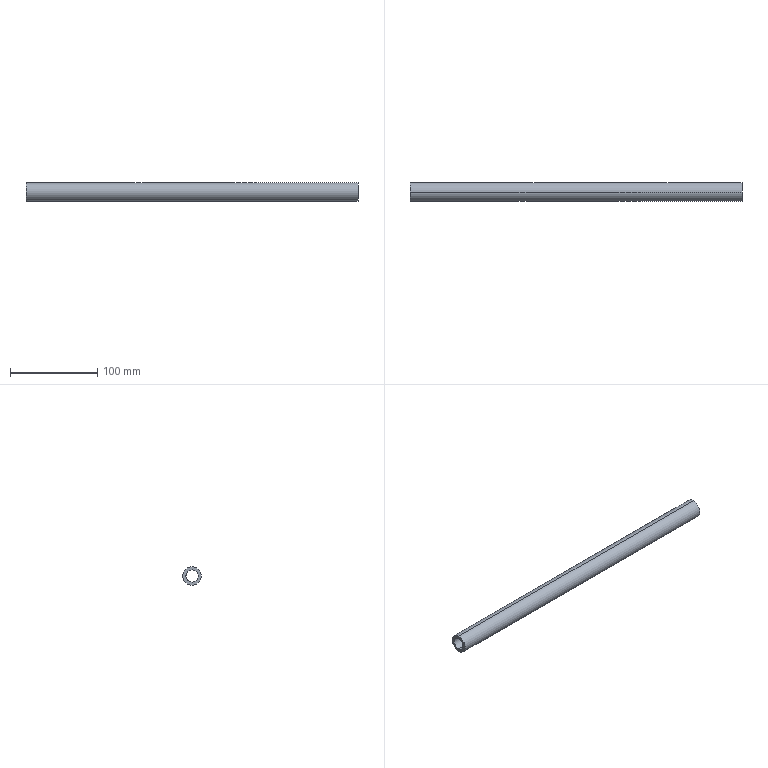Part | SolidWorks | features BaseBody 1, ICE 1 | 1 solid | 22 faces | box 381 x 21.235 x 21.234 mm | volume 75088 mm3 | cylinder 12 | plane 10 | commonest cylinder face diameters 10 x8 14 x2 21.234 x2